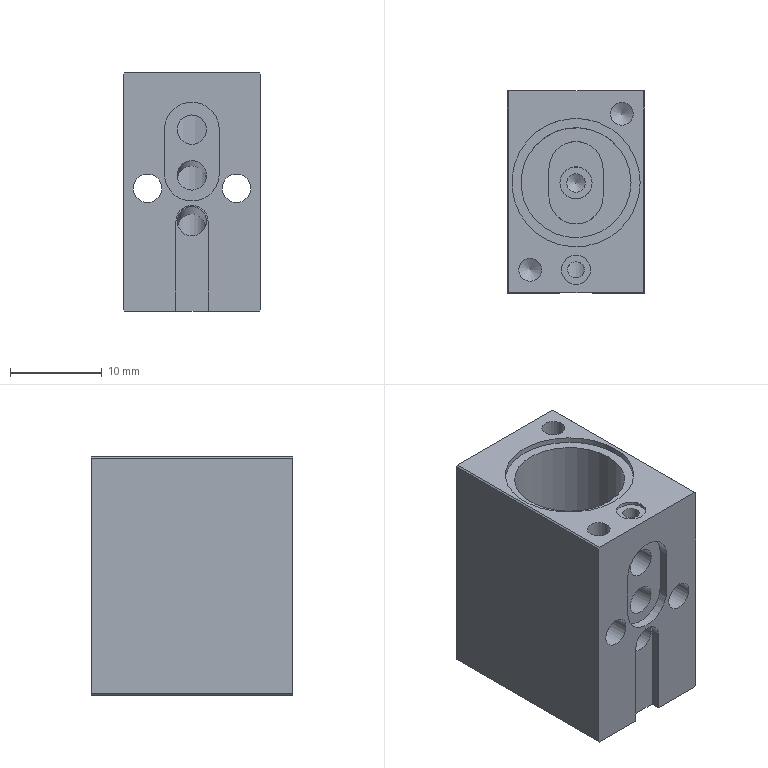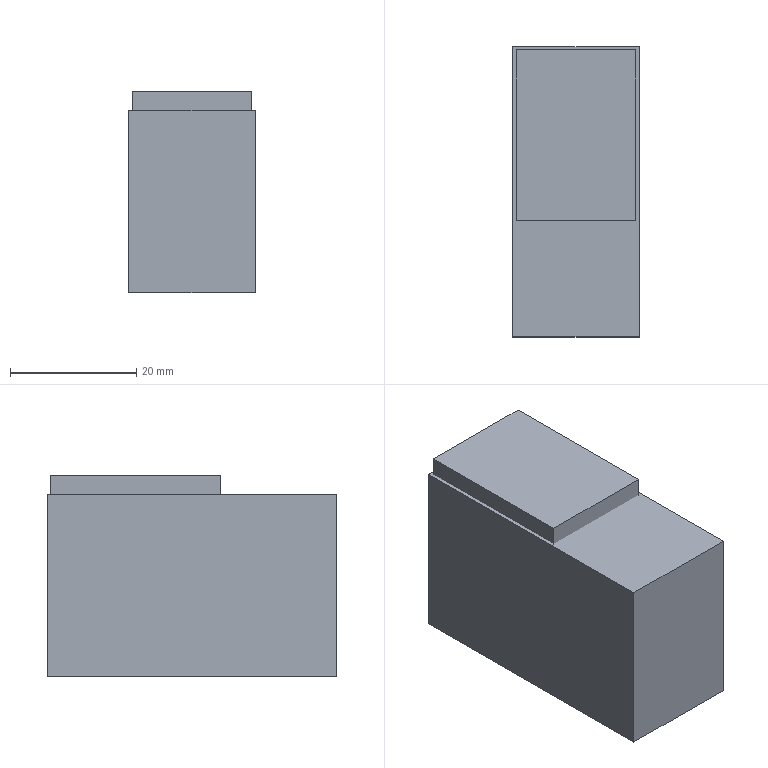CAM job | NX | 3+2 milling, 5-axis milling, drilling | part box 15 x 22 x 26 mm | stock box 20 x 46 x 32 mm
Tools:
number,name,description,diameter,corner_radius,flute_length,length,flutes
6,D3点钻,定心钻D4,3.0,0.0,43.0,75.0,2
2,D4点钻,定心钻D4,4.0,0.0,43.0,75.0,2
11,D2精光,D2,2.0,0.0,6.0,50.0,2
14,D3开粗,D3,3.0,0.0,9.0,50.0,2
5,D3精光,D3,3.0,0.0,9.0,50.0,2
13,D8开粗,D8,8.0,0.0,24.0,60.0,2
1,D8精光,D8,8.0,0.0,24.0,60.0,2
9,Z5.5,Z5.5直柄钻头,5.5,0.0,57.0,93.0,2
12,D50面刀,Milling Tool-5 Parameters,50.0,0.0,50.0,75.0,2
3,D3.1钻头,Drilling Tool,3.1,0.0,35.0,50.0,2
4,D3.2钻头,Drilling Tool,3.2,0.0,35.0,50.0,2
8,D2.3钻头,Drilling Tool,2.3,0.0,35.0,50.0,2
10,M2.5丝攻,Drilling Tool,2.5,0.0,35.0,50.0,2
7,D1.8钻头,Drilling Tool,1.8,0.0,35.0,50.0,2
15,R0.5,Milling Tool-Ball Mill,1.0,0.5,50.0,75.0,2
15,D2.8钻头,Drilling Tool,2.8,0.0,35.0,50.0,2
16,成型刀,Drilling Tool,2.0,0.0,35.0,50.0,2
0,D2R0.5,Milling Tool-5 Parameters,2.0,0.5,50.0,75.0,2
Operations:
program,operation,operation_type,tool,method,geometry_group,spindle_rpm,surface_speed,feed_per_tooth,feed_cut,feed_plunge,cut_length_mm,path_length_mm,cut_time_min,machine_time_min
XX-CNC1,PLANAR_MILL,PlanarMilling,D50面刀,METHOD,MCS_1,3500.0,100.0,0.1178,800.0,100.0,108.0,163.96,0.135,0.1406
XX-CNC1,PLANAR_MILL_COPY,PlanarMilling,D50面刀,METHOD,MCS_1,3500.0,549.0,0.0571,400.0,100.0,108.0,164.0,0.27,0.2756
XX-CNC1,ADAPTIVE_MILLING,CavityMilling,D8开粗,METHOD,W1,5500.0,138.0,0.2727,3000.0,100.0,955.308,1053.308,0.3108,0.3206
XX-CNC1,PLANAR_MILL_1,PlanarMilling,D8精光,METHOD,W1,5000.0,125.0,0.06,600.0,100.0,233.216,438.441,0.3887,0.4092
XX-CNC1,PLANAR_MILL_2,PlanarMilling,D3开粗,METHOD,W1,4500.0,100.0,0.1178,800.0,100.0,144.649,205.149,0.1808,0.1869
XX-CNC1,PLANAR_MILL_3,PlanarMilling,D3开粗,METHOD,W1,4500.0,100.0,0.1178,800.0,100.0,93.214,265.414,0.1165,0.1337
XX-CNC1,DRILLING,Operation,D4点钻,METHOD,W1,3000.0,0.0,0.0,200.0,0.0,9.2,91.553,0.046,0.0542
XX-CNC1,DRILLING_COPY,Operation,D4点钻,METHOD,W1,3000.0,0.0,0.0,200.0,0.0,4.7,71.4,0.0235,0.0302
XX-CNC1,DRILLING_COPY_1,Operation,D3.1钻头,METHOD,W1,3000.0,0.0,0.0,200.0,0.0,56.0,185.153,0.28,0.2929
XX-CNC1,DRILLING_COPY_COPY,Operation,D3.2钻头,METHOD,W1,3000.0,0.0,0.0,200.0,0.0,11.0,84.0,0.055,0.0623
XX-CNC2,DRILLING_1,Operation,D3开粗,METHOD,MCS_2,3000.0,0.0,0.0,100.0,0.0,4.0,11.0,0.04,0.0407
XX-CNC2,DRILLING_1_COPY,Operation,D3开粗,METHOD,MCS_2,3000.0,0.0,0.0,100.0,0.0,4.0,11.0,0.04,0.0407
XX-CNC2,DRILLING_1_COPY_1,Operation,D3点钻,METHOD,MCS_2,3000.0,0.0,0.0,200.0,0.0,4.5,12.0,0.0225,0.0233
XX-CNC2,DRILLING_1_COPY_COPY,Operation,D3点钻,METHOD,MCS_2,3000.0,0.0,0.0,200.0,0.0,4.5,12.0,0.0225,0.0233
XX-CNC2,DRILLING_1_COPY_1_COPY,Operation,D3.2钻头,METHOD,MCS_2,3000.0,0.0,0.0,200.0,0.0,12.0,27.0,0.06,0.0615
XX-CNC2,DRILLING_1_COPY_COPY_COPY,Operation,D3.2钻头,METHOD,MCS_2,3000.0,0.0,0.0,200.0,0.0,15.0,33.0,0.075,0.0768
XX-CNC2,3_AXIS_DEBURRING,TpMultiAxisDeburring,R0.5,METHOD,MCS_2,3000.0,0.0,0.0,270.0,90.0,32,58.854,0.1191,0.1191
XX-CNC3,DRILLING_2,Operation,D4点钻,METHOD,MCS_3,3000.0,0.0,0.0,200.0,0.0,17.0,136.303,0.085,0.0969
XX-CNC3,DRILLING_2_COPY_2,Operation,D1.8钻头,METHOD,MCS_3,3000.0,0.0,0.0,200.0,0.0,9.5,79.0,0.0475,0.0544
XX-CNC3,DRILLING_2_COPY_1,Operation,D2.3钻头,METHOD,MCS_3,3000.0,0.0,0.0,200.0,0.0,22.0,126.95,0.11,0.1205
XX-CNC3,DRILLING_2_COPY,Operation,Z5.5,METHOD,MCS_3,3000.0,0.0,0.0,200.0,0.0,17.0,94.0,0.085,0.0927
XX-CNC3,DRILLING_2_COPY_1_COPY,Operation,M2.5丝攻,METHOD,MCS_3,300.0,0.0,0.0,0.45,0.0,20.6,124.15,45.778,45.788
XX-CNC3,PLANAR_MILL_6,PlanarMilling,D8开粗,METHOD,MCS_3,4500.0,100.0,0.1178,1000.0,100.0,591.65,658.75,0.5917,0.5984
XX-CNC3,PLANAR_MILL_8,PlanarMilling,D8开粗,METHOD,MCS_3,4500.0,100.0,0.1178,600.0,100.0,31.091,88.091,0.0518,0.0575
XX-CNC3,PLANAR_MILL_7,PlanarMilling,D3开粗,METHOD,MCS_3,5500.0,100.0,0.1178,600.0,100.0,755.933,834.783,1.26,1.268
XX-CNC3,PLANAR_MILL_9,PlanarMilling,D8精光,METHOD,MCS_3,5500.0,100.0,0.1178,300.0,100.0,61.068,118.268,0.2036,0.2093
XX-CNC3,PLANAR_MILL_9_COPY,PlanarMilling,D8精光,METHOD,MCS_3,5500.0,138.0,0.0273,300.0,100.0,40.146,114.546,0.1338,0.1413
XX-CNC3,PLANAR_MILL_7_COPY,PlanarMilling,D3精光,METHOD,MCS_3,5500.0,100.0,0.1178,300.0,100.0,22.138,105.418,0.0738,0.0821
XX-CNC3,PLANAR_MILL_7_COPY_COPY,PlanarMilling,D3精光,METHOD,MCS_3,5500.0,100.0,0.1178,300.0,100.0,43.635,126.915,0.1454,0.1538
XX-CNC3,PLANAR_MILL_10,PlanarMilling,D2精光,METHOD,MCS_3,4500.0,100.0,0.0333,300.0,100.0,28.563,87.913,0.0952,0.1011
XX-CNC3,PLANAR_MILL_11,PlanarMilling,D3点钻,METHOD,MCS_3,4500.0,100.0,0.1178,800.0,100.0,60.819,184.902,0.076,0.0884
XX-CNC3,CURVE_DRIVE,SurfaceContour,D2R0.5,METHOD,MCS_3,4500.0,28.0,0.1111,1000.0,100.0,397.3,451.758,0.3973,0.4027
XX-CNC3,CURVE_DRIVE_COPY,SurfaceContour,D2R0.5,METHOD,MCS_3,4500.0,28.0,0.1111,1000.0,100.0,252.391,311.172,0.2524,0.2583
XX-CNC3,DRILLING_3,Operation,D1.8钻头,METHOD,MCS_3,3000.0,16.0,0.02,120.0,0.0,14.0,115.4,0.1167,0.1268
XX-CNC3,DRILLING_3_COPY,Operation,D2.8钻头,METHOD,MCS_3,3000.0,16.0,0.02,120.0,0.0,10.5,108.4,0.0875,0.0973
XX-CNC3,DRILLING_3_COPY_1,Operation,成型刀,METHOD,MCS_3,3000.0,16.0,0.02,40.0,0.0,14.15,115.7,0.3538,0.3639
XX-CNC4,PLANAR_MILL_13,PlanarMilling,D8开粗,METHOD,MCS_4,5500.0,138.0,0.0909,1000.0,100.0,126.0,354.0,0.126,0.1488
XX-CNC4,ADAPTIVE_MILLING_1,CavityMilling,D8开粗,METHOD,W4,5500.0,138.0,0.2727,3000.0,100.0,773.59,827.59,0.2579,0.2633
XX-CNC4,PLANAR_MILL_14,PlanarMilling,D50面刀,METHOD,MCS_4,4000.0,628.0,0.1,800.0,100.0,86.0,142.0,0.1075,0.1131
XX-CNC4,PLANAR_MILL_15,PlanarMilling,D3点钻,METHOD,MCS_4,4500.0,42.0,0.1111,1000.0,100.0,95.6,153.6,0.0956,0.1014
XX-CNC4,PLANAR_MILL_16,PlanarMilling,D3点钻,METHOD,MCS_4,4500.0,42.0,0.0667,600.0,100.0,17.612,143.346,0.0294,0.0419
XX-CNC5,PLANAR_MILL_2_COPY,PlanarMilling,D3精光,METHOD,W1,3000.0,100.0,0.05,300.0,100.0,27.552,85.512,0.0918,0.0976
XX-CNC5,PLANAR_MILL_2_COPY_COPY,PlanarMilling,D3精光,METHOD,W1,3000.0,100.0,0.05,300.0,100.0,30.737,88.697,0.1025,0.1083
XX-CNC5,PLANAR_MILL_3_COPY,PlanarMilling,D3精光,METHOD,W1,3000.0,100.0,0.05,300.0,100.0,31.385,89.385,0.1046,0.1104
XX-CNC5,PLANAR_MILL_4,PlanarMilling,D3点钻,METHOD,W1,4000.0,100.0,0.1178,1000.0,100.0,112.642,169.842,0.1126,0.1184
XX-CNC5,PLANAR_MILL_5,PlanarMilling,D3点钻,METHOD,W1,4000.0,100.0,0.1178,1000.0,100.0,32.135,89.335,0.0321,0.0379